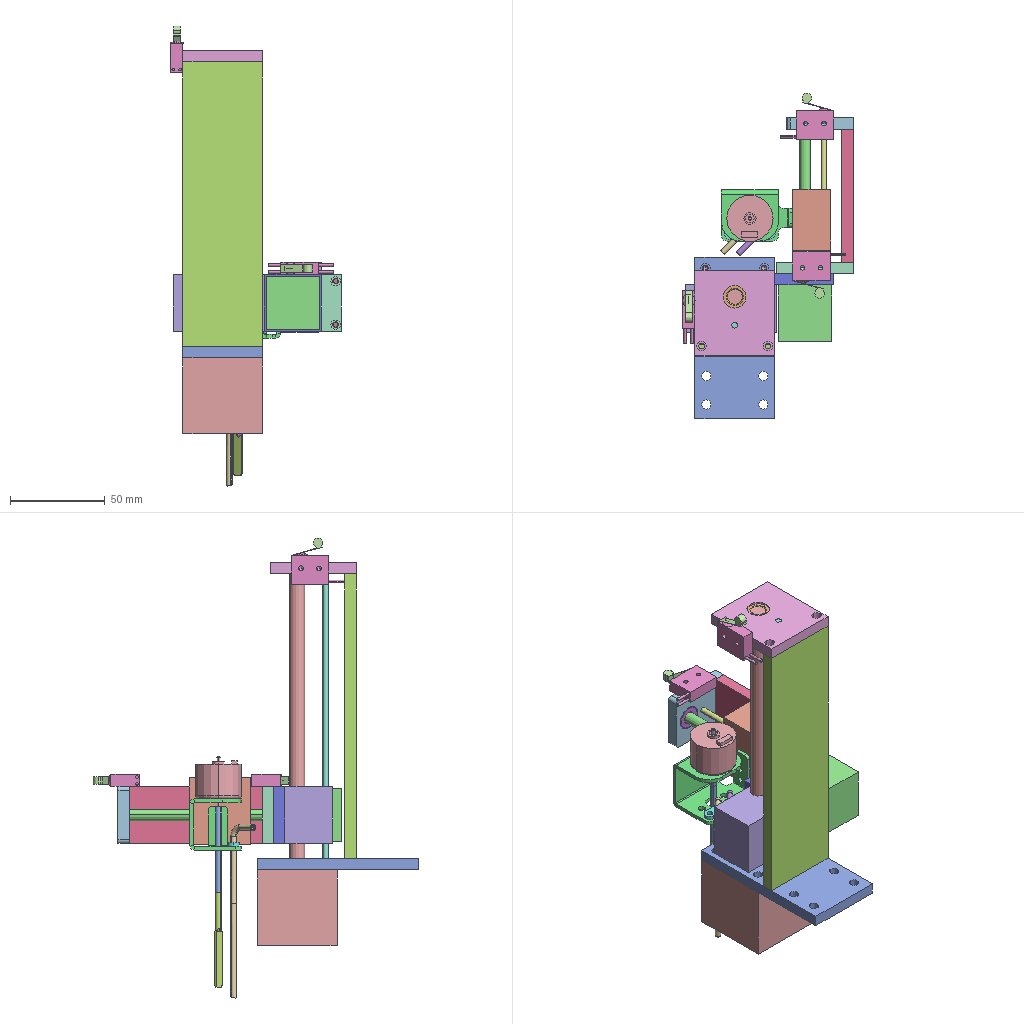Assembly | SolidWorks | 18 different items | 20 placed | box 90 x 171 x 242 mm
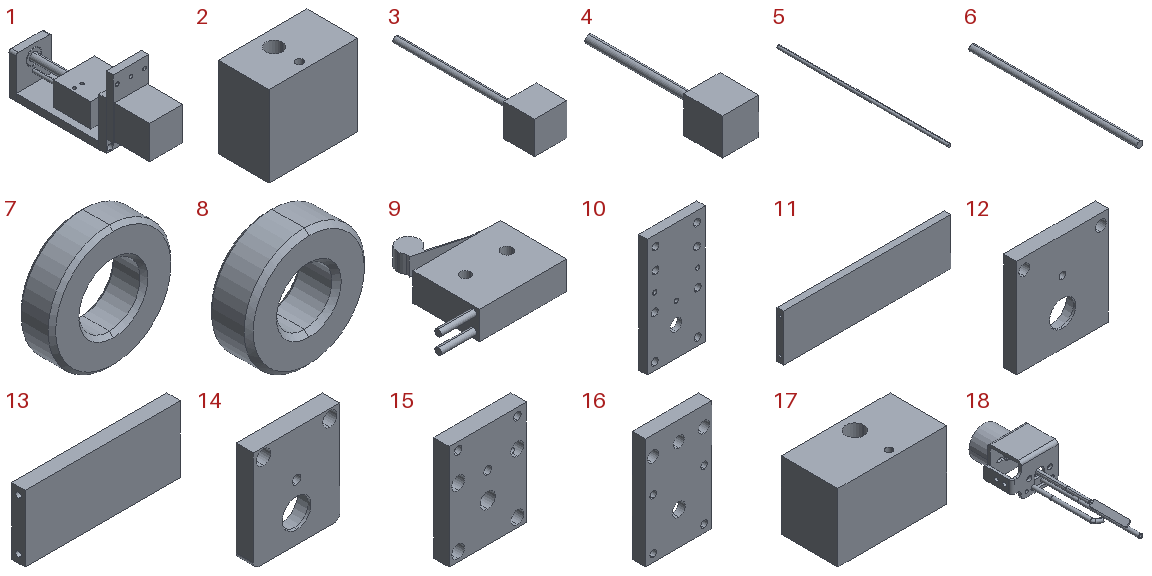Parts list (item | name | quantity | parent item | size | volume | features):
1 | (subassembly) | x1 | - | 35 x 118 x 60.5 mm | 80289 mm3 | -
2 | - | x1 | in 1 | 35 x 20 x 32 mm | 21036 mm3 | features Cut 2, Extrusion 1, HoleWzd 1
3 | - | x1 | - | 42 x 201 x 42 mm | 79160 mm3 | features ICE 3, Extrusion 1, HoleWzd 1
4 | - | x1 | in 1 | 28 x 117 x 28 mm | 26125 mm3 | features ICE 3, Extrusion 1, HoleWzd 1
5 | - | x1 | - | 3 x 162 x 3 mm | 1145 mm3 | features Extrusion 1
6 | - | x1 | in 1 | 3 x 82 x 3 mm | 579.624 mm3 | features Extrusion 1
7 | - | x1 | - | 16 x 4.5 x 16 mm | 659.734 mm3 | features Chamfer 1, Extrusion 1
8 | - | x1 | in 1 | 13 x 4.5 x 13 mm | 455.138 mm3 | features Chamfer 1, Extrusion 1
9 | - | x3 | - | 27.9 x 24.5 x 6.5 mm | 2034 mm3 | features BaseBody 2
10 | - | x1 | - | 42 x 6 x 85 mm | 19158 mm3 | features ICE 5, Cut 3, FlatPattern 1, SMBaseFlange 1, SheetMetal 1
11 | - | x1 | - | 150 x 6 x 42 mm | 37648 mm3 | features Cut 2, HoleWzd 2, Extrusion 1
12 | - | x1 | - | 42 x 6 x 45 mm | 9918 mm3 | features ICE 3, Cut 1, Extrusion 1, HoleWzd 1
13 | - | x1 | in 1 | 70 x 6 x 30 mm | 12502 mm3 | features Cut 2, Extrusion 1
14 | - | x1 | in 1 | 30 x 6 x 35 mm | 5244 mm3 | features ICE 4, Cut 2, Extrusion 1, HoleWzd 1
15 | - | x1 | in 1 | 30 x 6 x 40.5 mm | 6447 mm3 | features Cut 3, ICE 3, FlatPattern 1, HoleWzd 1, SMBaseFlange 1, SheetMetal 1
16 | - | x1 | in 1 | 30 x 6 x 50 mm | 7901 mm3 | features ICE 3, Cut 2, FlatPattern 1, SMBaseFlange 1, SheetMetal 1
17 | - | x1 | - | 48 x 25 x 30 mm | 34166 mm3 | features Cut 2, Extrusion 1, HoleWzd 1
18 | - | x1 | - | 37.96 x 127.1 x 34.667 mm | 14532 mm3 | features BaseBody 7
Mates (type | each side: item.copy, entity, surface, feature):
In the top assembly
Coincident | 3.1 face plane Boss-Extrude1 | 10.1 face plane Base-Flange1
Concentric | 3.1 face cylinder Boss-Extrude2 | 10.1 face cylinder Cut-Extrude2
Concentric | 3.1 face cylinder M3 Tapped Hole1 | 10.1 face cylinder Cut-Extrude3
Coincident | 10.1 face plane Base-Flange1 | 11.1 face plane Boss-Extrude1
DistanceDim | 3.1 face plane Boss-Extrude1 | 11.1 face plane Boss-Extrude1
Concentric | 10.1 face cylinder Cut-Extrude1 | 5.1 face cylinder Boss-Extrude1
Coincident | 3.1 face plane Boss-Extrude1 | 5.1 face plane Boss-Extrude1
Concentric | 3.1 face cylinder Boss-Extrude3 | 17.1 face cylinder Cut-Extrude2
Concentric | 5.1 face cylinder Boss-Extrude1 | 17.1 face cylinder Cut-Extrude2
Coincident | 11.1 face plane Boss-Extrude1 | 12.1 face plane Boss-Extrude1
Coincident | 12.1 face plane Cut-Extrude1 | 7.1 face plane Boss-Extrude1
Concentric | 12.1 face cylinder Cut-Extrude1 | 7.1 face cylinder Boss-Extrude1
Concentric | 3.1 face cylinder Boss-Extrude3 | 7.1 face cylinder Boss-Extrude1
Coincident | 17.1 face plane Boss-Extrude1 | 16.1 face plane Base-Flange1 | 2 times
DistanceDim | 17.1 face plane Boss-Extrude1 | 4.1 face plane Boss-Extrude1
Coincident | 14.1 face plane Boss-Extrude1 | 9.1 face plane Input2
Concentric | 14.1 face cylinder M3 Tapped Hole1 | 9.1 face cylinder Input2 | 2 times
Coincident | 12.1 face plane Boss-Extrude1 | 9.2 face plane Input2
Concentric | 12.1 face cylinder M3 Tapped Hole1 | 9.2 face cylinder Input2 | 2 times
Coincident | 15.1 face plane Base-Flange1 | 9.3 face plane Input2
Concentric | 15.1 face cylinder M3 Tapped Hole1 | 9.3 face cylinder Input2 | 2 times
Coincident | 2.1 face plane Boss-Extrude1 | 18.1 face plane
Concentric | 2.1 face cylinder M3 Tapped Hole1 | 18.1 face cylinder | 2 times
In subassembly 1
Concentric | 4.2 face cylinder Boss-Extrude3 | 14.2 face cylinder Cut-Extrude1
Coincident | 13.1 face plane Boss-Extrude1 | 14.2 face plane Boss-Extrude1 | 2 times
Concentric | 14.2 face cylinder Boss-Extrude1 | 6.1 face cylinder Boss-Extrude1
Coincident | 14.2 face plane Boss-Extrude1 | 6.1 face plane Boss-Extrude1
Coincident | 14.2 face plane Boss-Extrude1 | 8.1 face plane Boss-Extrude1
Concentric | 4.2 face cylinder Boss-Extrude3 | 8.1 face cylinder Boss-Extrude1
DistanceDim | 4.2 face plane Boss-Extrude1 | 15.2 face plane Base-Flange1
Concentric | 4.2 face cylinder Boss-Extrude3 | 15.2 face cylinder Cut-Extrude1
Concentric | 4.2 face cylinder M3 Tapped Hole1 | 15.2 face cylinder Cut-Extrude1
Concentric | 13.1 face cylinder Cut-Extrude1 | 14.2 face cylinder Cut-Extrude3
Concentric | 13.1 face cylinder Cut-Extrude1 | 14.2 face cylinder Cut-Extrude2
Coincident | 13.1 face plane Boss-Extrude1 | 15.2 face plane Base-Flange1
Coincident | 14.2 face plane Boss-Extrude1 | 15.2 face plane Base-Flange1
Concentric | 4.2 face cylinder Boss-Extrude3 | 2.2 face cylinder Cut-Extrude2
Concentric | 6.1 face cylinder Boss-Extrude1 | 2.2 face cylinder Cut-Extrude2
Coincident | 4.2 face plane Boss-Extrude1 | 16.2 face plane Base-Flange1
Concentric | 4.2 face cylinder Boss-Extrude3 | 16.2 face cylinder Cut-Extrude1
Coincident | 15.2 face plane Base-Flange1 | 16.2 face plane Base-Flange1